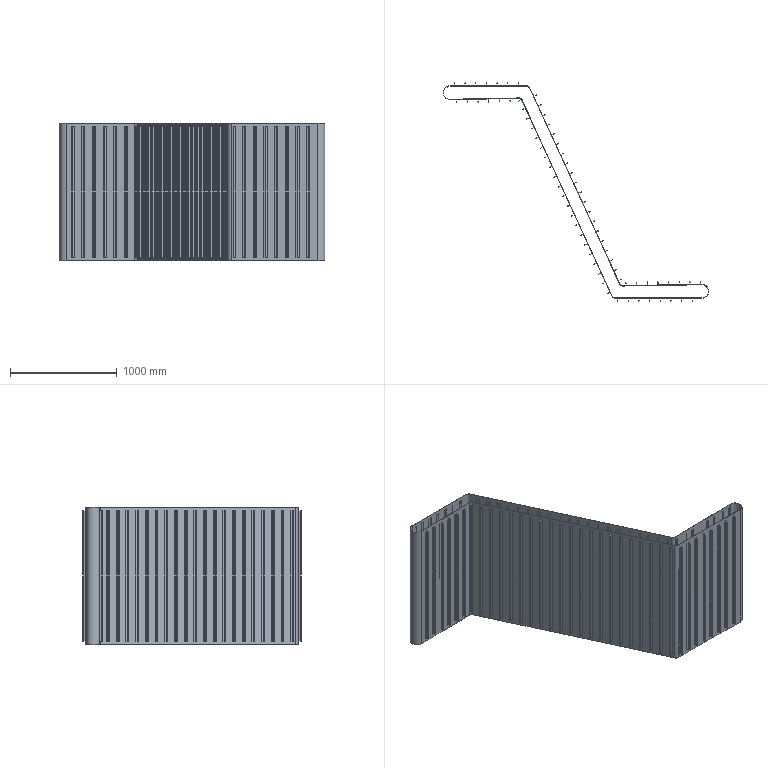Part | STEP file | Belt1-5^Produce dryer-Z conveyor | 1 solid | 619 faces | box 2487 x 2048 x 1290 mm | volume 28033863 mm3 | plane 605 | cylinder 14 | commonest cylinder face diameters 124 x3 128 x3 60 x2 64 x2 73 x2 77 x2